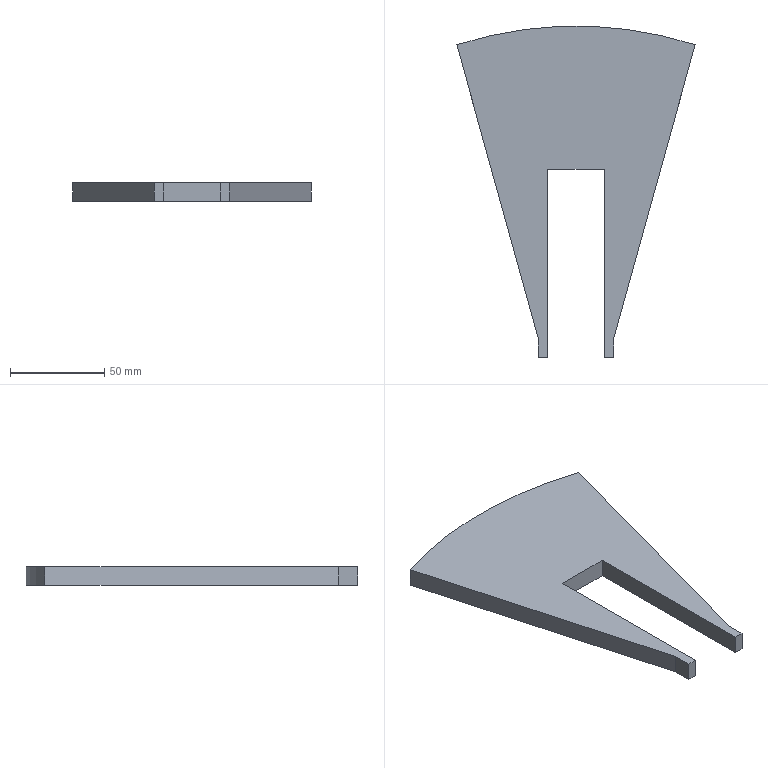Part | SolidWorks | features Extrusion 1, ICE 1 | 1 solid | 12 faces | box 126.548 x 176 x 10 mm | volume 112385 mm3 | plane 11 | cylinder 1 | commonest cylinder face diameters 412 x1
STEP:
#1=CARTESIAN_POINT('',(-20.,30.,-5.));
#2=VERTEX_POINT('',#1);
#3=CARTESIAN_POINT('',(-15.,30.,-5.));
#4=VERTEX_POINT('',#3);
#5=CARTESIAN_POINT('',(-20.,30.,-5.));
#6=DIRECTION('',(1.,0.,0.));
#7=VECTOR('',#6,1000.);
#8=LINE('',#5,#7);
#9=EDGE_CURVE('',#2,#4,#8,.T.);
#10=ORIENTED_EDGE('',*,*,#9,.T.);
#11=CARTESIAN_POINT('',(-15.,30.,5.));
#12=VERTEX_POINT('',#11);
#13=CARTESIAN_POINT('',(-15.,30.,5.));
#14=DIRECTION('',(0.,0.,1.));
#15=VECTOR('',#14,1000.);
#16=LINE('',#13,#15);
#17=EDGE_CURVE('',#4,#12,#16,.T.);
#18=ORIENTED_EDGE('',*,*,#17,.T.);
#19=CARTESIAN_POINT('',(-20.,30.,5.));
#20=VERTEX_POINT('',#19);
#21=CARTESIAN_POINT('',(-20.,30.,5.));
#22=DIRECTION('',(1.,0.,0.));
#23=VECTOR('',#22,1000.);
#24=LINE('',#21,#23);
#25=EDGE_CURVE('',#20,#12,#24,.T.);
#26=ORIENTED_EDGE('',*,*,#25,.F.);
#27=CARTESIAN_POINT('',(-20.,30.,5.));
#28=DIRECTION('',(0.,0.,-1.));
#29=VECTOR('',#28,1000.);
#30=LINE('',#27,#29);
#31=EDGE_CURVE('',#20,#2,#30,.T.);
#32=ORIENTED_EDGE('',*,*,#31,.T.);
#33=EDGE_LOOP('',(#10,#18,#26,#32));
#34=FACE_OUTER_BOUND('',#33,.T.);
#35=CARTESIAN_POINT('',(-20.,30.,5.));
#36=DIRECTION('',(0.,1.,0.));
#37=DIRECTION('',(0.,0.,1.));
#38=AXIS2_PLACEMENT_3D('',#35,#36,#37);
#39=PLANE('',#38);
#40=ADVANCED_FACE('',(#34),#39,.F.);
#41=CARTESIAN_POINT('',(63.274,196.042,-5.));
#42=VERTEX_POINT('',#41);
#43=CARTESIAN_POINT('',(-63.274,196.042,-5.));
#44=VERTEX_POINT('',#43);
#45=CARTESIAN_POINT('',(0.,0.,-5.));
#46=DIRECTION('',(0.,0.,1.));
#47=DIRECTION('',(1.,0.,0.));
#48=AXIS2_PLACEMENT_3D('',#45,#46,#47);
#49=CIRCLE('',#48,206.);
#50=EDGE_CURVE('',#42,#44,#49,.T.);
#51=ORIENTED_EDGE('',*,*,#50,.T.);
#52=CARTESIAN_POINT('',(-63.274,196.042,5.));
#53=VERTEX_POINT('',#52);
#54=CARTESIAN_POINT('',(-63.274,196.042,5.));
#55=DIRECTION('',(0.,0.,-1.));
#56=VECTOR('',#55,1000.);
#57=LINE('',#54,#56);
#58=EDGE_CURVE('',#53,#44,#57,.T.);
#59=ORIENTED_EDGE('',*,*,#58,.F.);
#60=CARTESIAN_POINT('',(63.274,196.042,5.));
#61=VERTEX_POINT('',#60);
#62=CARTESIAN_POINT('',(0.,0.,5.));
#63=DIRECTION('',(0.,0.,1.));
#64=DIRECTION('',(1.,0.,0.));
#65=AXIS2_PLACEMENT_3D('',#62,#63,#64);
#66=CIRCLE('',#65,206.);
#67=EDGE_CURVE('',#61,#53,#66,.T.);
#68=ORIENTED_EDGE('',*,*,#67,.F.);
#69=CARTESIAN_POINT('',(63.274,196.042,5.));
#70=DIRECTION('',(0.,0.,-1.));
#71=VECTOR('',#70,1000.);
#72=LINE('',#69,#71);
#73=EDGE_CURVE('',#61,#42,#72,.T.);
#74=ORIENTED_EDGE('',*,*,#73,.T.);
#75=EDGE_LOOP('',(#51,#59,#68,#74));
#76=FACE_OUTER_BOUND('',#75,.T.);
#77=CARTESIAN_POINT('',(0.,0.,5.));
#78=DIRECTION('',(0.,0.,-1.));
#79=DIRECTION('',(-1.,0.,0.));
#80=AXIS2_PLACEMENT_3D('',#77,#78,#79);
#81=CYLINDRICAL_SURFACE('',#80,206.);
#82=ADVANCED_FACE('',(#76),#81,.T.);
#83=CARTESIAN_POINT('',(-20.,40.,-5.));
#84=VERTEX_POINT('',#83);
#85=CARTESIAN_POINT('',(-63.274,196.042,-5.));
#86=DIRECTION('',(0.2672,-0.9636,0.));
#87=VECTOR('',#86,1000.);
#88=LINE('',#85,#87);
#89=EDGE_CURVE('',#44,#84,#88,.T.);
#90=ORIENTED_EDGE('',*,*,#89,.T.);
#91=CARTESIAN_POINT('',(-20.,40.,5.));
#92=VERTEX_POINT('',#91);
#93=CARTESIAN_POINT('',(-20.,40.,5.));
#94=DIRECTION('',(0.,0.,-1.));
#95=VECTOR('',#94,1000.);
#96=LINE('',#93,#95);
#97=EDGE_CURVE('',#92,#84,#96,.T.);
#98=ORIENTED_EDGE('',*,*,#97,.F.);
#99=CARTESIAN_POINT('',(-63.274,196.042,5.));
#100=DIRECTION('',(0.2672,-0.9636,0.));
#101=VECTOR('',#100,1000.);
#102=LINE('',#99,#101);
#103=EDGE_CURVE('',#53,#92,#102,.T.);
#104=ORIENTED_EDGE('',*,*,#103,.F.);
#105=ORIENTED_EDGE('',*,*,#58,.T.);
#106=EDGE_LOOP('',(#90,#98,#104,#105));
#107=FACE_OUTER_BOUND('',#106,.T.);
#108=CARTESIAN_POINT('',(-63.274,196.042,5.));
#109=DIRECTION('',(0.9636,0.2672,0.));
#110=DIRECTION('',(-0.2672,0.9636,0.));
#111=AXIS2_PLACEMENT_3D('',#108,#109,#110);
#112=PLANE('',#111);
#113=ADVANCED_FACE('',(#107),#112,.F.);
#114=CARTESIAN_POINT('',(-20.,40.,-5.));
#115=DIRECTION('',(0.,-1.,0.));
#116=VECTOR('',#115,1000.);
#117=LINE('',#114,#116);
#118=EDGE_CURVE('',#84,#2,#117,.T.);
#119=ORIENTED_EDGE('',*,*,#118,.T.);
#120=ORIENTED_EDGE('',*,*,#31,.F.);
#121=CARTESIAN_POINT('',(-20.,40.,5.));
#122=DIRECTION('',(0.,-1.,0.));
#123=VECTOR('',#122,1000.);
#124=LINE('',#121,#123);
#125=EDGE_CURVE('',#92,#20,#124,.T.);
#126=ORIENTED_EDGE('',*,*,#125,.F.);
#127=ORIENTED_EDGE('',*,*,#97,.T.);
#128=EDGE_LOOP('',(#119,#120,#126,#127));
#129=FACE_OUTER_BOUND('',#128,.T.);
#130=CARTESIAN_POINT('',(-20.,40.,5.));
#131=DIRECTION('',(1.,0.,0.));
#132=DIRECTION('',(0.,0.,-1.));
#133=AXIS2_PLACEMENT_3D('',#130,#131,#132);
#134=PLANE('',#133);
#135=ADVANCED_FACE('',(#129),#134,.F.);
#136=CARTESIAN_POINT('',(15.,30.,5.));
#137=VERTEX_POINT('',#136);
#138=CARTESIAN_POINT('',(20.,30.,5.));
#139=VERTEX_POINT('',#138);
#140=CARTESIAN_POINT('',(-20.,30.,5.));
#141=DIRECTION('',(1.,0.,0.));
#142=VECTOR('',#141,1000.);
#143=LINE('',#140,#142);
#144=EDGE_CURVE('',#137,#139,#143,.T.);
#145=ORIENTED_EDGE('',*,*,#144,.F.);
#146=CARTESIAN_POINT('',(15.,30.,-5.));
#147=VERTEX_POINT('',#146);
#148=CARTESIAN_POINT('',(15.,30.,5.));
#149=DIRECTION('',(0.,0.,-1.));
#150=VECTOR('',#149,1000.);
#151=LINE('',#148,#150);
#152=EDGE_CURVE('',#137,#147,#151,.T.);
#153=ORIENTED_EDGE('',*,*,#152,.T.);
#154=CARTESIAN_POINT('',(20.,30.,-5.));
#155=VERTEX_POINT('',#154);
#156=CARTESIAN_POINT('',(-20.,30.,-5.));
#157=DIRECTION('',(1.,0.,0.));
#158=VECTOR('',#157,1000.);
#159=LINE('',#156,#158);
#160=EDGE_CURVE('',#147,#155,#159,.T.);
#161=ORIENTED_EDGE('',*,*,#160,.T.);
#162=CARTESIAN_POINT('',(20.,30.,5.));
#163=DIRECTION('',(0.,0.,-1.));
#164=VECTOR('',#163,1000.);
#165=LINE('',#162,#164);
#166=EDGE_CURVE('',#139,#155,#165,.T.);
#167=ORIENTED_EDGE('',*,*,#166,.F.);
#168=EDGE_LOOP('',(#145,#153,#161,#167));
#169=FACE_OUTER_BOUND('',#168,.T.);
#170=CARTESIAN_POINT('',(-20.,30.,5.));
#171=DIRECTION('',(0.,1.,0.));
#172=DIRECTION('',(0.,0.,1.));
#173=AXIS2_PLACEMENT_3D('',#170,#171,#172);
#174=PLANE('',#173);
#175=ADVANCED_FACE('',(#169),#174,.F.);
#176=CARTESIAN_POINT('',(20.,40.,-5.));
#177=VERTEX_POINT('',#176);
#178=CARTESIAN_POINT('',(20.,30.,-5.));
#179=DIRECTION('',(0.,1.,0.));
#180=VECTOR('',#179,1000.);
#181=LINE('',#178,#180);
#182=EDGE_CURVE('',#155,#177,#181,.T.);
#183=ORIENTED_EDGE('',*,*,#182,.T.);
#184=CARTESIAN_POINT('',(20.,40.,5.));
#185=VERTEX_POINT('',#184);
#186=CARTESIAN_POINT('',(20.,40.,5.));
#187=DIRECTION('',(0.,0.,-1.));
#188=VECTOR('',#187,1000.);
#189=LINE('',#186,#188);
#190=EDGE_CURVE('',#185,#177,#189,.T.);
#191=ORIENTED_EDGE('',*,*,#190,.F.);
#192=CARTESIAN_POINT('',(20.,30.,5.));
#193=DIRECTION('',(0.,1.,0.));
#194=VECTOR('',#193,1000.);
#195=LINE('',#192,#194);
#196=EDGE_CURVE('',#139,#185,#195,.T.);
#197=ORIENTED_EDGE('',*,*,#196,.F.);
#198=ORIENTED_EDGE('',*,*,#166,.T.);
#199=EDGE_LOOP('',(#183,#191,#197,#198));
#200=FACE_OUTER_BOUND('',#199,.T.);
#201=CARTESIAN_POINT('',(20.,30.,5.));
#202=DIRECTION('',(-1.,0.,0.));
#203=DIRECTION('',(0.,-1.,0.));
#204=AXIS2_PLACEMENT_3D('',#201,#202,#203);
#205=PLANE('',#204);
#206=ADVANCED_FACE('',(#200),#205,.F.);
#207=CARTESIAN_POINT('',(20.,40.,-5.));
#208=DIRECTION('',(0.2672,0.9636,0.));
#209=VECTOR('',#208,1000.);
#210=LINE('',#207,#209);
#211=EDGE_CURVE('',#177,#42,#210,.T.);
#212=ORIENTED_EDGE('',*,*,#211,.T.);
#213=ORIENTED_EDGE('',*,*,#73,.F.);
#214=CARTESIAN_POINT('',(20.,40.,5.));
#215=DIRECTION('',(0.2672,0.9636,0.));
#216=VECTOR('',#215,1000.);
#217=LINE('',#214,#216);
#218=EDGE_CURVE('',#185,#61,#217,.T.);
#219=ORIENTED_EDGE('',*,*,#218,.F.);
#220=ORIENTED_EDGE('',*,*,#190,.T.);
#221=EDGE_LOOP('',(#212,#213,#219,#220));
#222=FACE_OUTER_BOUND('',#221,.T.);
#223=CARTESIAN_POINT('',(20.,40.,5.));
#224=DIRECTION('',(-0.9636,0.2672,0.));
#225=DIRECTION('',(-0.2672,-0.9636,0.));
#226=AXIS2_PLACEMENT_3D('',#223,#224,#225);
#227=PLANE('',#226);
#228=ADVANCED_FACE('',(#222),#227,.F.);
#229=CARTESIAN_POINT('',(-15.,130.,5.));
#230=VERTEX_POINT('',#229);
#231=CARTESIAN_POINT('',(-15.,-70.,5.));
#232=DIRECTION('',(0.,-1.,0.));
#233=VECTOR('',#232,1000.);
#234=LINE('',#231,#233);
#235=EDGE_CURVE('',#230,#12,#234,.T.);
#236=ORIENTED_EDGE('',*,*,#235,.F.);
#237=CARTESIAN_POINT('',(15.,130.,5.));
#238=VERTEX_POINT('',#237);
#239=CARTESIAN_POINT('',(15.,130.,5.));
#240=DIRECTION('',(-1.,0.,0.));
#241=VECTOR('',#240,1000.);
#242=LINE('',#239,#241);
#243=EDGE_CURVE('',#238,#230,#242,.T.);
#244=ORIENTED_EDGE('',*,*,#243,.F.);
#245=CARTESIAN_POINT('',(15.,-70.,5.));
#246=DIRECTION('',(0.,1.,0.));
#247=VECTOR('',#246,1000.);
#248=LINE('',#245,#247);
#249=EDGE_CURVE('',#137,#238,#248,.T.);
#250=ORIENTED_EDGE('',*,*,#249,.F.);
#251=ORIENTED_EDGE('',*,*,#144,.T.);
#252=ORIENTED_EDGE('',*,*,#196,.T.);
#253=ORIENTED_EDGE('',*,*,#218,.T.);
#254=ORIENTED_EDGE('',*,*,#67,.T.);
#255=ORIENTED_EDGE('',*,*,#103,.T.);
#256=ORIENTED_EDGE('',*,*,#125,.T.);
#257=ORIENTED_EDGE('',*,*,#25,.T.);
#258=EDGE_LOOP('',(#236,#244,#250,#251,#252,#253,#254,#255,#256,#257));
#259=FACE_OUTER_BOUND('',#258,.T.);
#260=CARTESIAN_POINT('',(0.,0.,5.));
#261=DIRECTION('',(0.,0.,1.));
#262=DIRECTION('',(1.,0.,0.));
#263=AXIS2_PLACEMENT_3D('',#260,#261,#262);
#264=PLANE('',#263);
#265=ADVANCED_FACE('',(#259),#264,.T.);
#266=CARTESIAN_POINT('',(15.,130.,-5.));
#267=VERTEX_POINT('',#266);
#268=CARTESIAN_POINT('',(-15.,130.,-5.));
#269=VERTEX_POINT('',#268);
#270=CARTESIAN_POINT('',(15.,130.,-5.));
#271=DIRECTION('',(-1.,0.,0.));
#272=VECTOR('',#271,1000.);
#273=LINE('',#270,#272);
#274=EDGE_CURVE('',#267,#269,#273,.T.);
#275=ORIENTED_EDGE('',*,*,#274,.T.);
#276=CARTESIAN_POINT('',(-15.,-70.,-5.));
#277=DIRECTION('',(0.,-1.,0.));
#278=VECTOR('',#277,1000.);
#279=LINE('',#276,#278);
#280=EDGE_CURVE('',#269,#4,#279,.T.);
#281=ORIENTED_EDGE('',*,*,#280,.T.);
#282=ORIENTED_EDGE('',*,*,#9,.F.);
#283=ORIENTED_EDGE('',*,*,#118,.F.);
#284=ORIENTED_EDGE('',*,*,#89,.F.);
#285=ORIENTED_EDGE('',*,*,#50,.F.);
#286=ORIENTED_EDGE('',*,*,#211,.F.);
#287=ORIENTED_EDGE('',*,*,#182,.F.);
#288=ORIENTED_EDGE('',*,*,#160,.F.);
#289=CARTESIAN_POINT('',(15.,0.,-5.));
#290=DIRECTION('',(0.,1.,0.));
#291=VECTOR('',#290,1000.);
#292=LINE('',#289,#291);
#293=EDGE_CURVE('',#147,#267,#292,.T.);
#294=ORIENTED_EDGE('',*,*,#293,.T.);
#295=EDGE_LOOP('',(#275,#281,#282,#283,#284,#285,#286,#287,#288,#294));
#296=FACE_OUTER_BOUND('',#295,.T.);
#297=CARTESIAN_POINT('',(0.,0.,-5.));
#298=DIRECTION('',(0.,0.,1.));
#299=DIRECTION('',(1.,0.,0.));
#300=AXIS2_PLACEMENT_3D('',#297,#298,#299);
#301=PLANE('',#300);
#302=ADVANCED_FACE('',(#296),#301,.F.);
#303=ORIENTED_EDGE('',*,*,#280,.F.);
#304=CARTESIAN_POINT('',(-15.,130.,-5.));
#305=DIRECTION('',(0.,0.,1.));
#306=VECTOR('',#305,1000.);
#307=LINE('',#304,#306);
#308=EDGE_CURVE('',#269,#230,#307,.T.);
#309=ORIENTED_EDGE('',*,*,#308,.T.);
#310=ORIENTED_EDGE('',*,*,#235,.T.);
#311=ORIENTED_EDGE('',*,*,#17,.F.);
#312=EDGE_LOOP('',(#303,#309,#310,#311));
#313=FACE_OUTER_BOUND('',#312,.T.);
#314=CARTESIAN_POINT('',(-15.,-70.,-5.));
#315=DIRECTION('',(-1.,0.,0.));
#316=DIRECTION('',(0.,0.,1.));
#317=AXIS2_PLACEMENT_3D('',#314,#315,#316);
#318=PLANE('',#317);
#319=ADVANCED_FACE('',(#313),#318,.F.);
#320=ORIENTED_EDGE('',*,*,#249,.T.);
#321=CARTESIAN_POINT('',(15.,130.,-5.));
#322=DIRECTION('',(0.,0.,1.));
#323=VECTOR('',#322,1000.);
#324=LINE('',#321,#323);
#325=EDGE_CURVE('',#267,#238,#324,.T.);
#326=ORIENTED_EDGE('',*,*,#325,.F.);
#327=ORIENTED_EDGE('',*,*,#293,.F.);
#328=ORIENTED_EDGE('',*,*,#152,.F.);
#329=EDGE_LOOP('',(#320,#326,#327,#328));
#330=FACE_OUTER_BOUND('',#329,.T.);
#331=CARTESIAN_POINT('',(15.,-70.,-5.));
#332=DIRECTION('',(1.,0.,0.));
#333=DIRECTION('',(0.,0.,-1.));
#334=AXIS2_PLACEMENT_3D('',#331,#332,#333);
#335=PLANE('',#334);
#336=ADVANCED_FACE('',(#330),#335,.F.);
#337=ORIENTED_EDGE('',*,*,#243,.T.);
#338=ORIENTED_EDGE('',*,*,#308,.F.);
#339=ORIENTED_EDGE('',*,*,#274,.F.);
#340=ORIENTED_EDGE('',*,*,#325,.T.);
#341=EDGE_LOOP('',(#337,#338,#339,#340));
#342=FACE_OUTER_BOUND('',#341,.T.);
#343=CARTESIAN_POINT('',(15.,130.,-5.));
#344=DIRECTION('',(0.,1.,0.));
#345=DIRECTION('',(0.,0.,1.));
#346=AXIS2_PLACEMENT_3D('',#343,#344,#345);
#347=PLANE('',#346);
#348=ADVANCED_FACE('',(#342),#347,.F.);
#349=CLOSED_SHELL('',(#40,#82,#113,#135,#175,#206,#228,#265,#302,#319,#336,#348));
#350=MANIFOLD_SOLID_BREP('',#349);
#351=CARTESIAN_POINT('',(0.,0.,0.));
#352=DIRECTION('',(0.,0.,1.));
#353=DIRECTION('',(1.,0.,0.));
#354=AXIS2_PLACEMENT_3D('',#351,#352,#353);
#355=(LENGTH_UNIT()NAMED_UNIT(*)SI_UNIT(.MILLI.,.METRE.));
#356=UNCERTAINTY_MEASURE_WITH_UNIT(LENGTH_MEASURE(0.00001),#355,'','');
#357=(NAMED_UNIT(*)PLANE_ANGLE_UNIT()SI_UNIT($,.RADIAN.));
#358=(NAMED_UNIT(*)SI_UNIT($,.STERADIAN.)SOLID_ANGLE_UNIT());
#359=(GEOMETRIC_REPRESENTATION_CONTEXT(3)GLOBAL_UNCERTAINTY_ASSIGNED_CONTEXT((#356))GLOBAL_UNIT_ASSIGNED_CONTEXT((#355,#357,#358))REPRESENTATION_CONTEXT('',''));
#360=ADVANCED_BREP_SHAPE_REPRESENTATION('',(#350,#354),#359);